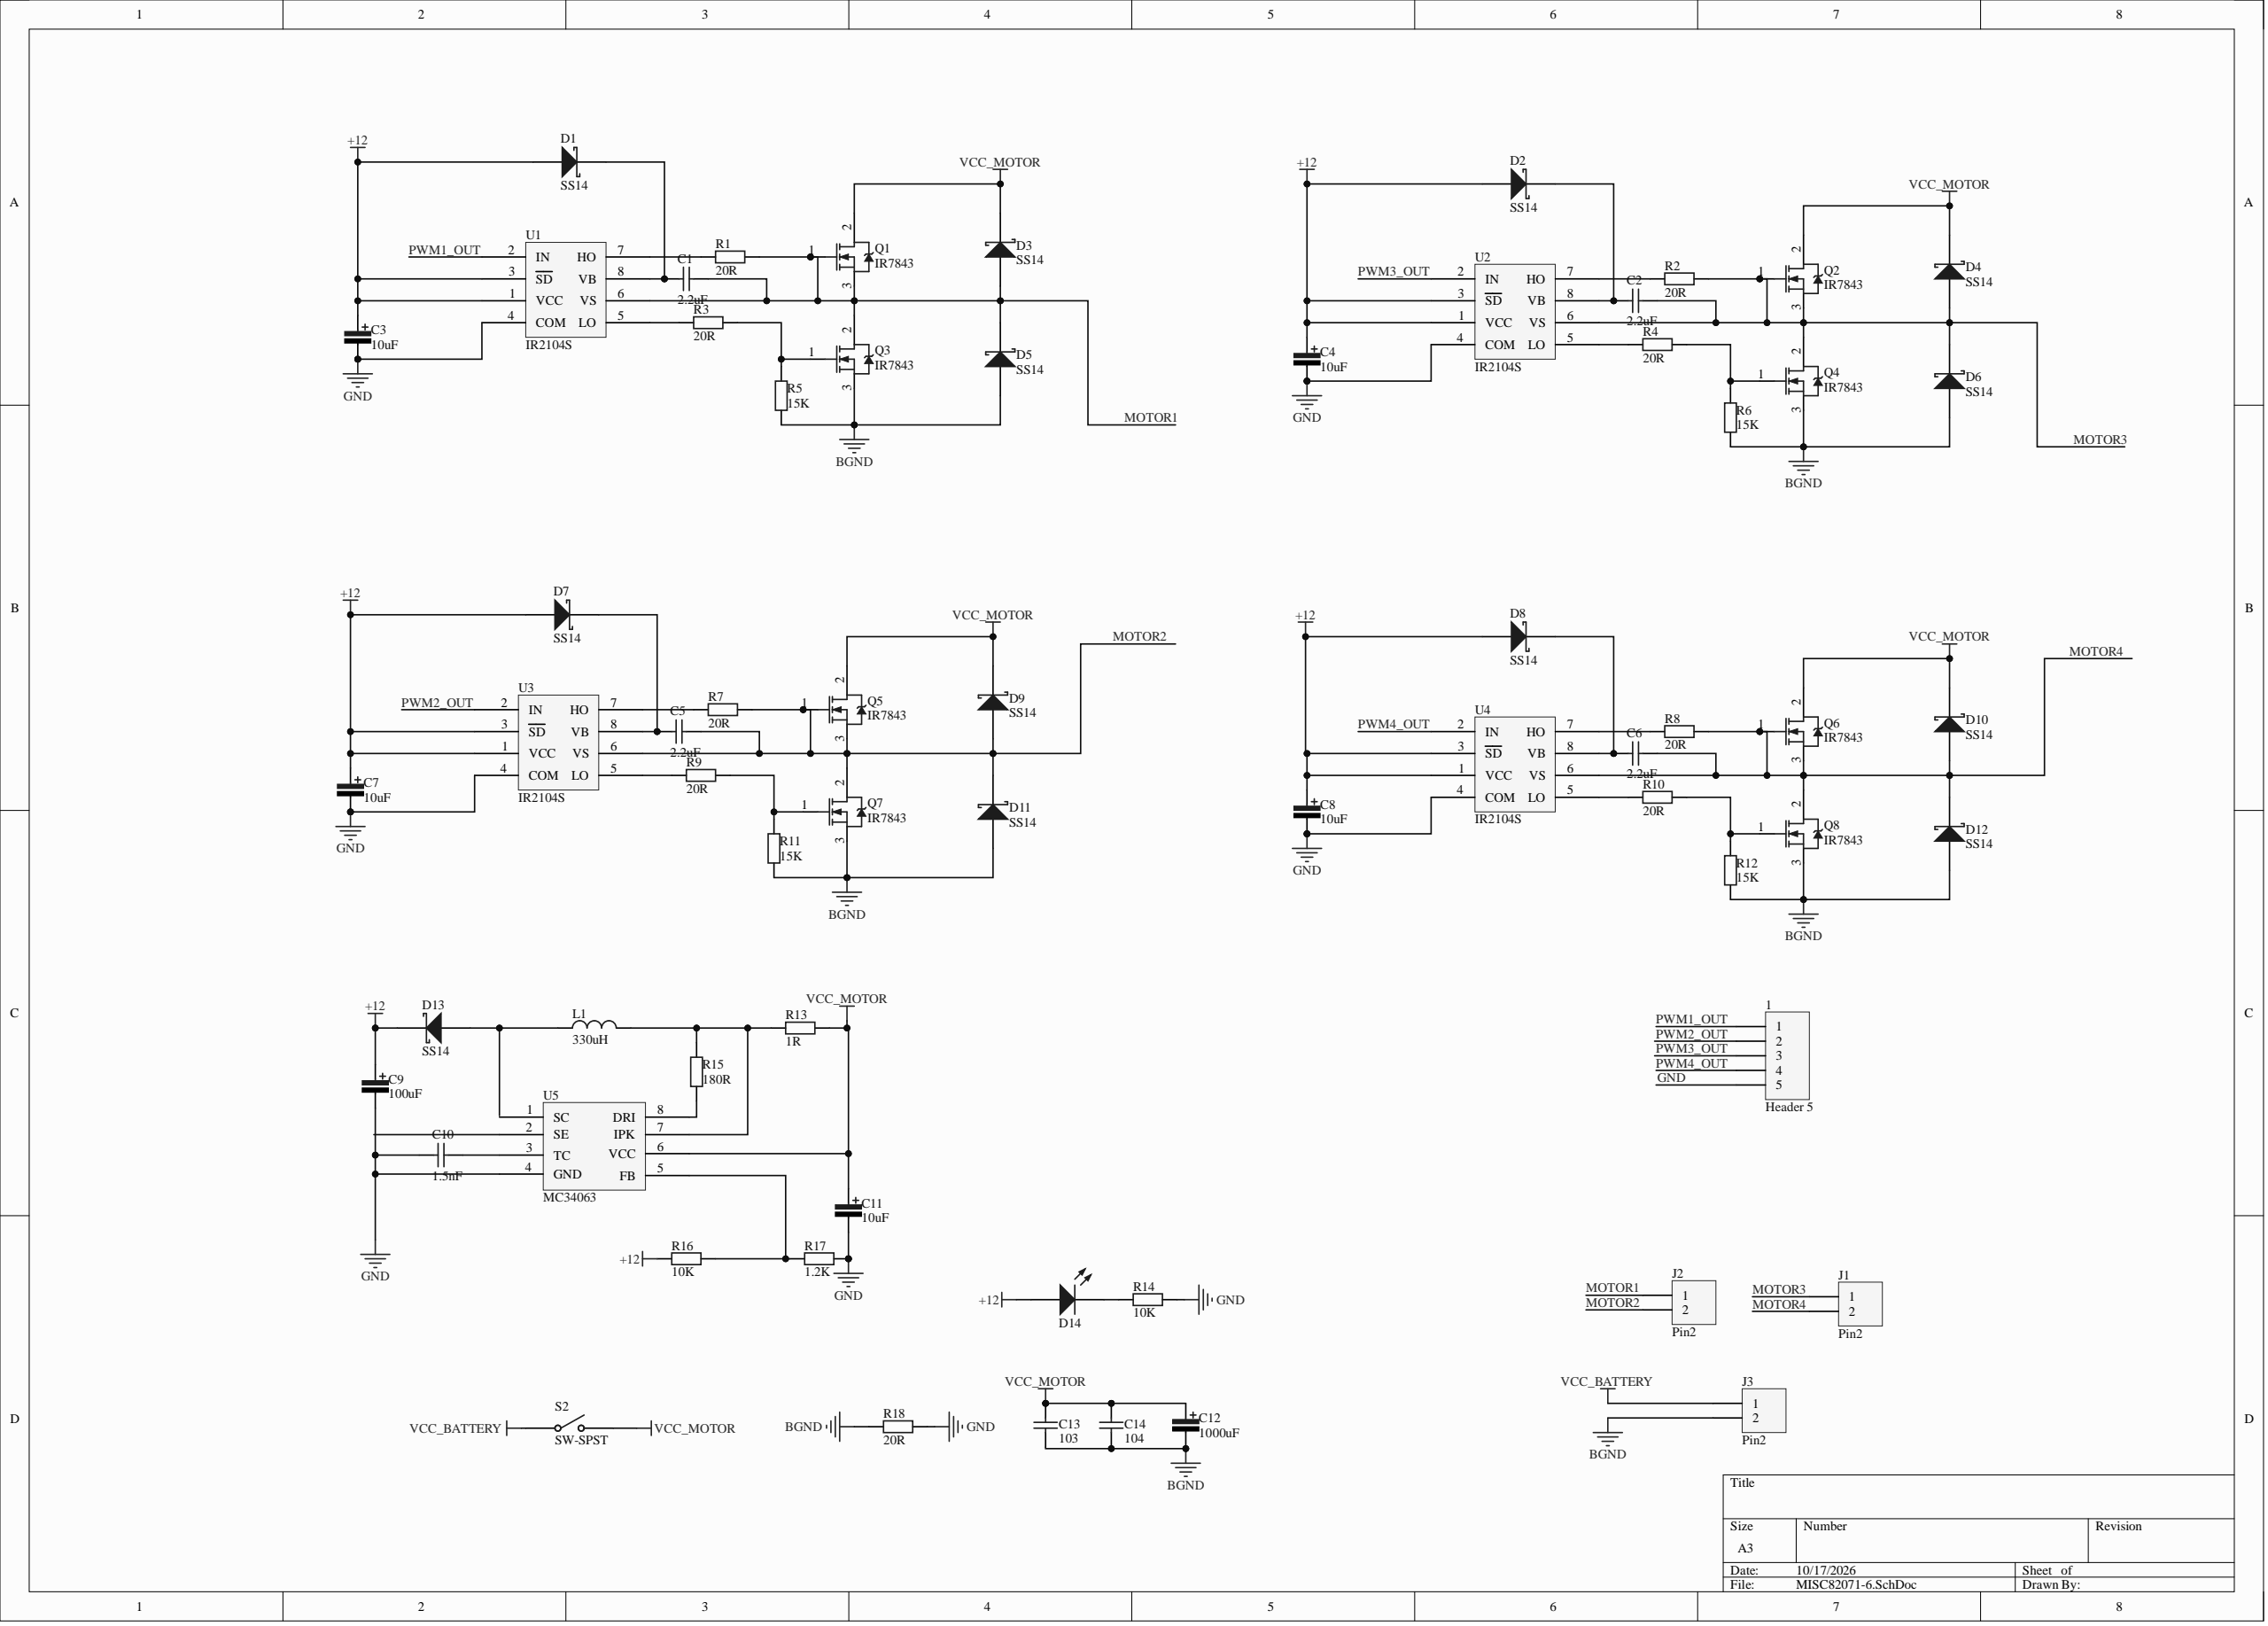Circuit board | Altium Designer | 65 parts | 35 nets
Bill of materials:
Comment,Description,Designator,Footprint,LibRef,Quantity
"Header 5","Header, 5-Pin","1","HDR1X5","Header 5","1"
"Cap","Non-polarized capacitor","C1, C2, C5, C6, C10, C13, C14","my0603","Cap","7"
"Cap Pol","Polarized electrolytic capacitor","C3, C4, C7, C8, C9, C11","CAP-3528","Cap Pol","6"
"Cap Pol","Polarized electrolytic capacitor","C12","CM A(3*5.4)","Cap Pol","1"
"D-Schottky","Schottky diode","D1, D2, D3, D4, D5, D6, D7, D8, D9, D10, D11, D12, D13","DIODE-SMA","D-Schottky","13"
"LED0","LED","D14","0805","LED0","1"
"Pin2","","J1, J2, J3","PCBComponent_1 - duplicate","Pin2","3"
"Inductor","Inductor","L1","L-SMD-7","Inductor","1"
"IR7843","N-Channel Power MOSFET","Q1, Q2, Q3, Q4, Q5, Q6, Q7, Q8","LR7843","NMOS","8"
"Res1","Chip resistor","R1, R2, R3, R4, R5, R6, R7, R8, R9, R10, R11, R12, R13, R14, R15, R16, R17, R18","0805","Res1","18"
"SW-SPST","Single-Pole, Single-Throw Switch","S2","SWITCH","SW-SPST","1"
"IR2104S","","U1, U2, U3, U4","IR2104","IR2104","4"
"MC34063","","U5","MC34063","MC34063","1"
Netlist (Protel format):
[
1
HDR1X5
Header 5



]
[
C1
my0603
Cap



]
[
C2
my0603
Cap



]
[
C3
CAP-3528
Cap Pol



]
[
C4
CAP-3528
Cap Pol



]
[
C5
my0603
Cap



]
[
C6
my0603
Cap



]
[
C7
CAP-3528
Cap Pol



]
[
C8
CAP-3528
Cap Pol



]
[
C9
CAP-3528
Cap Pol



]
[
C10
my0603
Cap



]
[
C11
CAP-3528
Cap Pol



]
[
C12
CM A(3*5.4)
Cap Pol



]
[
C13
my0603
Cap



]
[
C14
my0603
Cap



]
[
D1
DIODE-SMA
D-Schottky



]
[
D2
DIODE-SMA
D-Schottky



]
[
D3
DIODE-SMA
D-Schottky



]
[
D4
DIODE-SMA
D-Schottky



]
[
D5
DIODE-SMA
D-Schottky



]
[
D6
DIODE-SMA
D-Schottky



]
[
D7
DIODE-SMA
D-Schottky



]
[
D8
DIODE-SMA
D-Schottky



]
[
D9
DIODE-SMA
D-Schottky



]
[
D10
DIODE-SMA
D-Schottky



]
[
D11
DIODE-SMA
D-Schottky



]
[
D12
DIODE-SMA
D-Schottky



]
[
D13
DIODE-SMA
D-Schottky



]
[
D14
0805
LED0



]
[
J1
PCBComponent_1 - duplicate
Pin2



]
[
J2
PCBComponent_1 - duplicate
Pin2



]
[
J3
PCBComponent_1 - duplicate
Pin2



]
[
L1
L-SMD-7
Inductor



]
[
Q1
LR7843
IR7843



]
[
Q2
LR7843
IR7843



]
[
Q3
LR7843
IR7843



]
[
Q4
LR7843
IR7843



]
[
Q5
LR7843
IR7843



]
[
Q6
LR7843
IR7843



]
[
Q7
LR7843
IR7843



]
[
Q8
LR7843
IR7843



]
[
R1
0805
Res1



]
[
R2
0805
Res1



]
[
R3
0805
Res1



]
[
R4
0805
Res1



]
[
R5
0805
Res1



]
[
R6
0805
Res1



]
[
R7
0805
Res1



]
[
R8
0805
Res1



]
[
R9
0805
Res1



]
[
R10
0805
Res1



]
[
R11
0805
Res1



]
[
R12
0805
Res1



]
[
R13
0805
Res1



]
[
R14
0805
Res1



]
[
R15
0805
Res1



]
[
R16
0805
Res1



]
[
R17
0805
Res1



]
[
R18
0805
Res1



]
[
S2
SWITCH
SW-SPST



]
[
U1
IR2104
IR2104S



]
[
U2
IR2104
IR2104S



]
[
U3
IR2104
IR2104S



]
[
U4
IR2104
IR2104S



]
[
U5
MC34063
MC34063



]
(
VCC_MOTOR
C11-1
C12-1
C13-2
C14-2
D3-2
D4-2
D9-2
D10-2
Q1-2
Q2-2
Q5-2
Q6-2
R13-2
S2-2
U5-6
)
(
VCC_BATTERY
J3-1
S2-1
)
(
PWM4_OUT
1-4
U4-2
)
(
PWM3_OUT
1-3
U2-2
)
(
PWM2_OUT
1-2
U3-2
)
(
PWM1_OUT
1-1
U1-2
)
(
NetR16_2
R16-2
R17-1
U5-5
)
(
NetR15_1
R15-1
U5-8
)
(
NetR10_1
R10-1
U4-5
)
(
NetR9_1
R9-1
U3-5
)
(
NetR8_1
R8-1
U4-7
)
(
NetR7_1
R7-1
U3-7
)
(
NetR4_1
R4-1
U2-5
)
(
NetR3_1
R3-1
U1-5
)
(
NetR2_1
R2-1
U2-7
)
(
NetR1_1
R1-1
U1-7
)
(
NetQ8_1
Q8-1
R10-2
R12-2
)
(
NetQ7_1
Q7-1
R9-2
R11-2
)
(
NetQ4_1
Q4-1
R4-2
R6-2
)
(
NetQ3_1
Q3-1
R3-2
R5-2
)
(
NetL1_2
L1-2
R13-1
R15-2
U5-7
)
(
NetD14_2
D14-2
R14-1
)
(
NetD13_1
D13-1
L1-1
)
(
NetC10_2
C10-2
U5-3
)
(
NetC6_1
C6-1
D8-2
U4-8
)
(
NetC5_1
C5-1
D7-2
U3-8
)
(
NetC2_1
C2-1
D2-2
U2-8
)
(
NetC1_1
C1-1
D1-2
U1-8
)
(
MOTOR4
C6-2
D10-1
D12-2
J1-2
Q6-1
Q6-3
Q8-2
R8-2
U4-6
)
(
MOTOR3
C2-2
D4-1
D6-2
J1-1
Q2-1
Q2-3
Q4-2
R2-2
U2-6
)
(
MOTOR2
C5-2
D9-1
D11-2
J2-2
Q5-1
Q5-3
Q7-2
R7-2
U3-6
)
(
MOTOR1
C1-2
D3-1
D5-2
J2-1
Q1-1
Q1-3
Q3-2
R1-2
U1-6
)
(
GND
1-5
C3-2
C4-2
C7-2
C8-2
C9-2
C10-1
C11-2
R14-2
R17-2
R18-2
U1-4
U2-4
U3-4
U4-4
U5-4
)
(
BGND
C12-2
C13-1
C14-1
D5-1
D6-1
D11-1
D12-1
J3-2
Q3-3
Q4-3
Q7-3
Q8-3
R5-1
R6-1
R11-1
R12-1
R18-1
)
(
+12
C3-1
C4-1
C7-1
C8-1
C9-1
D1-1
D2-1
D7-1
D8-1
D13-2
D14-1
R16-1
U1-1
U1-3
U2-1
U2-3
U3-1
U3-3
U4-1
U4-3
)